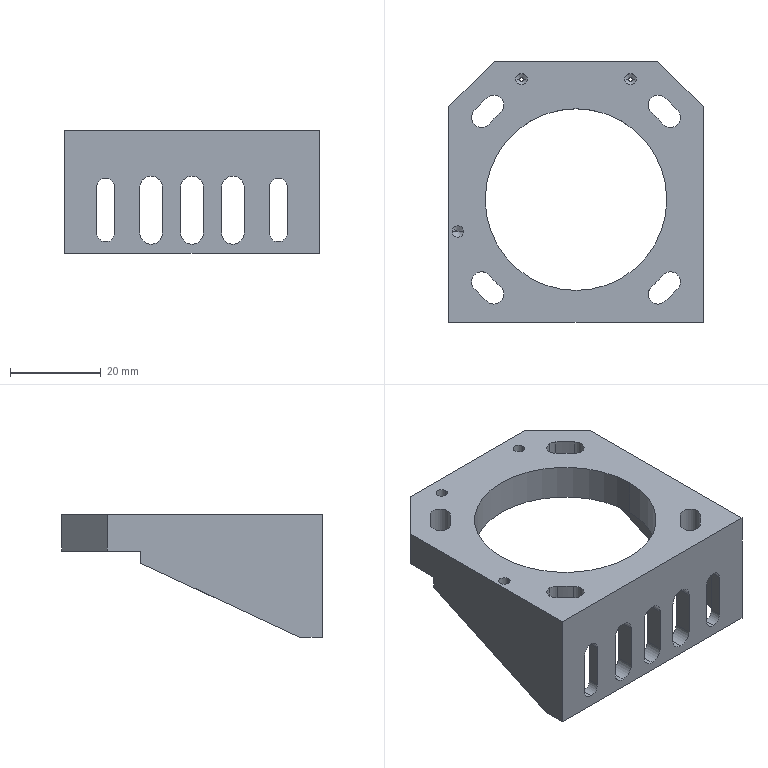NC program | NX | posted with a generic post | part box 56 x 57.4 x 27 mm
Lines 1 to 1144 of 3091:
N10 G17 G21 G94 G90
(ZLEVEL_PROFILE_COPY_1_COPY , TOOL : D3)
N12 T03 M6
N14 G54
N16 G17 G0 G90 X5.642 Y-19.45 B0. C0. S5500 M3
N18 G43 Z30. H3
N20 Z0.8
N22 G94 G1 X9.095 Z0.619 F1000.
N24 X9.326 Y-19.325 Z0.605
N26 X9.45 Y-19.094 Z0.592
N28 Y-18.903 Z0.582
N30 X9.325 Y-18.674 Z0.568
N32 X9.095 Y-18.55 Z0.554
N34 X-1.095 Z0.02
N36 X-1.225 Y-18.599 Z0.013
N38 X-1.335 Y-18.685 Z0.006
N40 X-1.434 Y-18.848 Z-0.004
N42 X-1.448 Y-19.105 Z-0.018
N44 X-1.32 Y-19.33 Z-0.032
N46 X-1.159 Y-19.432 Z-0.042
N48 X-1.095 Y-19.45 Z-0.045
N50 X-1. Z-0.05
N52 X9. F1250.
N54 G3 X9.45 Y-19. R0.45
N56 X9. Y-18.55 R0.45
N58 G1 X-1.
N60 G3 X-1.45 Y-19. R0.45
N62 X-1. Y-19.45 R0.45
N64 G1 X1.864 Z-0.1
N66 X9.
N68 G3 X9.45 Y-19. R0.45
N70 X9. Y-18.55 R0.45
N72 G1 X-1.
N74 G3 X-1.45 Y-19. R0.45
N76 X-1. Y-19.45 R0.45
N78 G1 X1.864 Z-0.15
N80 X9.
N82 G3 X9.45 Y-19. R0.45
N84 X9. Y-18.55 R0.45
N86 G1 X-1.
N88 G3 X-1.45 Y-19. R0.45
N90 X-1. Y-19.45 R0.45
N92 G1 X1.864 Z-0.2
N94 X9.
N96 G3 X9.45 Y-19. R0.45
N98 X9. Y-18.55 R0.45
N100 G1 X-1.
N102 G3 X-1.45 Y-19. R0.45
N104 X-1. Y-19.45 R0.45
N106 G1 X1.864 Z-0.25
N108 X9.
N110 G3 X9.45 Y-19. R0.45
N112 X9. Y-18.55 R0.45
N114 G1 X-1.
N116 G3 X-1.45 Y-19. R0.45
N118 X-1. Y-19.45 R0.45
N120 G1 X1.864 Z-0.3
N122 X9.
N124 G3 X9.45 Y-19. R0.45
N126 X9. Y-18.55 R0.45
N128 G1 X-1.
N130 G3 X-1.45 Y-19. R0.45
N132 X-1. Y-19.45 R0.45
N134 G1 X1.864 Z-0.35
N136 X9.
N138 G3 X9.45 Y-19. R0.45
N140 X9. Y-18.55 R0.45
N142 G1 X-1.
N144 G3 X-1.45 Y-19. R0.45
N146 X-1. Y-19.45 R0.45
N148 G1 X1.864 Z-0.4
N150 X9.
N152 G3 X9.45 Y-19. R0.45
N154 X9. Y-18.55 R0.45
N156 G1 X-1.
N158 G3 X-1.45 Y-19. R0.45
N160 X-1. Y-19.45 R0.45
N162 G1 X1.864 Z-0.45
N164 X9.
N166 G3 X9.45 Y-19. R0.45
N168 X9. Y-18.55 R0.45
N170 G1 X-1.
N172 G3 X-1.45 Y-19. R0.45
N174 X-1. Y-19.45 R0.45
N176 G1 X1.864 Z-0.5
N178 X9.
N180 G3 X9.45 Y-19. R0.45
N182 X9. Y-18.55 R0.45
N184 G1 X-1.
N186 G3 X-1.45 Y-19. R0.45
N188 X-1. Y-19.45 R0.45
N190 G1 X1.864 Z-0.55
N192 X9.
N194 G3 X9.45 Y-19. R0.45
N196 X9. Y-18.55 R0.45
N198 G1 X-1.
N200 G3 X-1.45 Y-19. R0.45
N202 X-1. Y-19.45 R0.45
N204 G1 X1.864 Z-0.6
N206 X9.
N208 G3 X9.45 Y-19. R0.45
N210 X9. Y-18.55 R0.45
N212 G1 X-1.
N214 G3 X-1.45 Y-19. R0.45
N216 X-1. Y-19.45 R0.45
N218 G1 X1.864 Z-0.65
N220 X9.
N222 G3 X9.45 Y-19. R0.45
N224 X9. Y-18.55 R0.45
N226 G1 X-1.
N228 G3 X-1.45 Y-19. R0.45
N230 X-1. Y-19.45 R0.45
N232 G1 X1.864 Z-0.7
N234 X9.
N236 G3 X9.45 Y-19. R0.45
N238 X9. Y-18.55 R0.45
N240 G1 X-1.
N242 G3 X-1.45 Y-19. R0.45
N244 X-1. Y-19.45 R0.45
N246 G1 X1.864 Z-0.75
N248 X9.
N250 G3 X9.45 Y-19. R0.45
N252 X9. Y-18.55 R0.45
N254 G1 X-1.
N256 G3 X-1.45 Y-19. R0.45
N258 X-1. Y-19.45 R0.45
N260 G1 X1.864 Z-0.8
N262 X9.
N264 G3 X9.45 Y-19. R0.45
N266 X9. Y-18.55 R0.45
N268 G1 X-1.
N270 G3 X-1.45 Y-19. R0.45
N272 X-1. Y-19.45 R0.45
N274 G1 X1.864 Z-0.85
N276 X9.
N278 G3 X9.45 Y-19. R0.45
N280 X9. Y-18.55 R0.45
N282 G1 X-1.
N284 G3 X-1.45 Y-19. R0.45
N286 X-1. Y-19.45 R0.45
N288 G1 X1.864 Z-0.9
N290 X9.
N292 G3 X9.45 Y-19. R0.45
N294 X9. Y-18.55 R0.45
N296 G1 X-1.
N298 G3 X-1.45 Y-19. R0.45
N300 X-1. Y-19.45 R0.45
N302 G1 X1.864 Z-0.95
N304 X9.
N306 G3 X9.45 Y-19. R0.45
N308 X9. Y-18.55 R0.45
N310 G1 X-1.
N312 G3 X-1.45 Y-19. R0.45
N314 X-1. Y-19.45 R0.45
N316 G1 X1.864 Z-1.
N318 X9.
N320 G3 X9.45 Y-19. R0.45
N322 X9. Y-18.55 R0.45
N324 G1 X-1.
N326 G3 X-1.45 Y-19. R0.45
N328 X-1. Y-19.45 R0.45
N330 G1 X1.864 Z-1.05
N332 X9.
N334 G3 X9.45 Y-19. R0.45
N336 X9. Y-18.55 R0.45
N338 G1 X-1.
N340 G3 X-1.45 Y-19. R0.45
N342 X-1. Y-19.45 R0.45
N344 G1 X1.864 Z-1.1
N346 X9.
N348 G3 X9.45 Y-19. R0.45
N350 X9. Y-18.55 R0.45
N352 G1 X-1.
N354 G3 X-1.45 Y-19. R0.45
N356 X-1. Y-19.45 R0.45
N358 G1 X1.864 Z-1.15
N360 X9.
N362 G3 X9.45 Y-19. R0.45
N364 X9. Y-18.55 R0.45
N366 G1 X-1.
N368 G3 X-1.45 Y-19. R0.45
N370 X-1. Y-19.45 R0.45
N372 G1 X1.864 Z-1.2
N374 X9.
N376 G3 X9.45 Y-19. R0.45
N378 X9. Y-18.55 R0.45
N380 G1 X-1.
N382 G3 X-1.45 Y-19. R0.45
N384 X-1. Y-19.45 R0.45
N386 G1 X1.864 Z-1.25
N388 X9.
N390 G3 X9.45 Y-19. R0.45
N392 X9. Y-18.55 R0.45
N394 G1 X-1.
N396 G3 X-1.45 Y-19. R0.45
N398 X-1. Y-19.45 R0.45
N400 G1 X1.864 Z-1.3
N402 X9.
N404 G3 X9.45 Y-19. R0.45
N406 X9. Y-18.55 R0.45
N408 G1 X-1.
N410 G3 X-1.45 Y-19. R0.45
N412 X-1. Y-19.45 R0.45
N414 G1 X1.864 Z-1.35
N416 X9.
N418 G3 X9.45 Y-19. R0.45
N420 X9. Y-18.55 R0.45
N422 G1 X-1.
N424 G3 X-1.45 Y-19. R0.45
N426 X-1. Y-19.45 R0.45
N428 G1 X1.864 Z-1.4
N430 X9.
N432 G3 X9.45 Y-19. R0.45
N434 X9. Y-18.55 R0.45
N436 G1 X-1.
N438 G3 X-1.45 Y-19. R0.45
N440 X-1. Y-19.45 R0.45
N442 G1 X1.864 Z-1.45
N444 X9.
N446 G3 X9.45 Y-19. R0.45
N448 X9. Y-18.55 R0.45
N450 G1 X-1.
N452 G3 X-1.45 Y-19. R0.45
N454 X-1. Y-19.45 R0.45
N456 G1 X1.864 Z-1.5
N458 X9.
N460 G3 X9.45 Y-19. R0.45
N462 X9. Y-18.55 R0.45
N464 G1 X-1.
N466 G3 X-1.45 Y-19. R0.45
N468 X-1. Y-19.45 R0.45
N470 G1 X1.864 Z-1.55
N472 X9.
N474 G3 X9.45 Y-19. R0.45
N476 X9. Y-18.55 R0.45
N478 G1 X-1.
N480 G3 X-1.45 Y-19. R0.45
N482 X-1. Y-19.45 R0.45
N484 G1 X1.864 Z-1.6
N486 X9.
N488 G3 X9.45 Y-19. R0.45
N490 X9. Y-18.55 R0.45
N492 G1 X-1.
N494 G3 X-1.45 Y-19. R0.45
N496 X-1. Y-19.45 R0.45
N498 G1 X1.864 Z-1.65
N500 X9.
N502 G3 X9.45 Y-19. R0.45
N504 X9. Y-18.55 R0.45
N506 G1 X-1.
N508 G3 X-1.45 Y-19. R0.45
N510 X-1. Y-19.45 R0.45
N512 G1 X1.864 Z-1.7
N514 X9.
N516 G3 X9.45 Y-19. R0.45
N518 X9. Y-18.55 R0.45
N520 G1 X-1.
N522 G3 X-1.45 Y-19. R0.45
N524 X-1. Y-19.45 R0.45
N526 G1 X1.864 Z-1.75
N528 X9.
N530 G3 X9.45 Y-19. R0.45
N532 X9. Y-18.55 R0.45
N534 G1 X-1.
N536 G3 X-1.45 Y-19. R0.45
N538 X-1. Y-19.45 R0.45
N540 G1 X1.864 Z-1.8
N542 X9.
N544 G3 X9.45 Y-19. R0.45
N546 X9. Y-18.55 R0.45
N548 G1 X-1.
N550 G3 X-1.45 Y-19. R0.45
N552 X-1. Y-19.45 R0.45
N554 G1 X1.864 Z-1.85
N556 X9.
N558 G3 X9.45 Y-19. R0.45
N560 X9. Y-18.55 R0.45
N562 G1 X-1.
N564 G3 X-1.45 Y-19. R0.45
N566 X-1. Y-19.45 R0.45
N568 G1 X1.864 Z-1.9
N570 X9.
N572 G3 X9.45 Y-19. R0.45
N574 X9. Y-18.55 R0.45
N576 G1 X-1.
N578 G3 X-1.45 Y-19. R0.45
N580 X-1. Y-19.45 R0.45
N582 G1 X1.864 Z-1.95
N584 X9.
N586 G3 X9.45 Y-19. R0.45
N588 X9. Y-18.55 R0.45
N590 G1 X-1.
N592 G3 X-1.45 Y-19. R0.45
N594 X-1. Y-19.45 R0.45
N596 G1 X1.864 Z-2.
N598 X9.
N600 G3 X9.45 Y-19. R0.45
N602 X9. Y-18.55 R0.45
N604 G1 X-1.
N606 G3 X-1.45 Y-19. R0.45
N608 X-1. Y-19.45 R0.45
N610 G1 X1.864 Z-2.05
N612 X9.
N614 G3 X9.45 Y-19. R0.45
N616 X9. Y-18.55 R0.45
N618 G1 X-1.
N620 G3 X-1.45 Y-19. R0.45
N622 X-1. Y-19.45 R0.45
N624 G1 X1.864 Z-2.1
N626 X9.
N628 G3 X9.45 Y-19. R0.45
N630 X9. Y-18.55 R0.45
N632 G1 X-1.
N634 G3 X-1.45 Y-19. R0.45
N636 X-1. Y-19.45 R0.45
N638 G1 X1.864 Z-2.15
N640 X9.
N642 G3 X9.45 Y-19. R0.45
N644 X9. Y-18.55 R0.45
N646 G1 X-1.
N648 G3 X-1.45 Y-19. R0.45
N650 X-1. Y-19.45 R0.45
N652 G1 X1.864 Z-2.2
N654 X9.
N656 G3 X9.45 Y-19. R0.45
N658 X9. Y-18.55 R0.45
N660 G1 X-1.
N662 G3 X-1.45 Y-19. R0.45
N664 X-1. Y-19.45 R0.45
N666 G1 X1.864 Z-2.25
N668 X9.
N670 G3 X9.45 Y-19. R0.45
N672 X9. Y-18.55 R0.45
N674 G1 X-1.
N676 G3 X-1.45 Y-19. R0.45
N678 X-1. Y-19.45 R0.45
N680 G1 X1.864 Z-2.3
N682 X9.
N684 G3 X9.45 Y-19. R0.45
N686 X9. Y-18.55 R0.45
N688 G1 X-1.
N690 G3 X-1.45 Y-19. R0.45
N692 X-1. Y-19.45 R0.45
N694 G1 X1.864 Z-2.35
N696 X9.
N698 G3 X9.45 Y-19. R0.45
N700 X9. Y-18.55 R0.45
N702 G1 X-1.
N704 G3 X-1.45 Y-19. R0.45
N706 X-1. Y-19.45 R0.45
N708 G1 X1.864 Z-2.4
N710 X9.
N712 G3 X9.45 Y-19. R0.45
N714 X9. Y-18.55 R0.45
N716 G1 X-1.
N718 G3 X-1.45 Y-19. R0.45
N720 X-1. Y-19.45 R0.45
N722 G1 X1.864 Z-2.45
N724 X9.
N726 G3 X9.45 Y-19. R0.45
N728 X9. Y-18.55 R0.45
N730 G1 X-1.
N732 G3 X-1.45 Y-19. R0.45
N734 X-1. Y-19.45 R0.45
N736 G1 X1.864 Z-2.5
N738 X9.
N740 G3 X9.45 Y-19. R0.45
N742 X9. Y-18.55 R0.45
N744 G1 X-1.
N746 G3 X-1.45 Y-19. R0.45
N748 X-1. Y-19.45 R0.45
N750 G1 X1.864 Z-2.55
N752 X9.
N754 G3 X9.45 Y-19. R0.45
N756 X9. Y-18.55 R0.45
N758 G1 X-1.
N760 G3 X-1.45 Y-19. R0.45
N762 X-1. Y-19.45 R0.45
N764 G1 X1.864 Z-2.6
N766 X9.
N768 G3 X9.45 Y-19. R0.45
N770 X9. Y-18.55 R0.45
N772 G1 X-1.
N774 G3 X-1.45 Y-19. R0.45
N776 X-1. Y-19.45 R0.45
N778 G1 X1.864 Z-2.65
N780 X9.
N782 G3 X9.45 Y-19. R0.45
N784 X9. Y-18.55 R0.45
N786 G1 X-1.
N788 G3 X-1.45 Y-19. R0.45
N790 X-1. Y-19.45 R0.45
N792 G1 X1.864 Z-2.7
N794 X9.
N796 G3 X9.45 Y-19. R0.45
N798 X9. Y-18.55 R0.45
N800 G1 X-1.
N802 G3 X-1.45 Y-19. R0.45
N804 X-1. Y-19.45 R0.45
N806 G1 X1.864 Z-2.75
N808 X9.
N810 G3 X9.45 Y-19. R0.45
N812 X9. Y-18.55 R0.45
N814 G1 X-1.
N816 G3 X-1.45 Y-19. R0.45
N818 X-1. Y-19.45 R0.45
N820 G1 X1.864 Z-2.8
N822 X9.
N824 G3 X9.45 Y-19. R0.45
N826 X9. Y-18.55 R0.45
N828 G1 X-1.
N830 G3 X-1.45 Y-19. R0.45
N832 X-1. Y-19.45 R0.45
N834 G1 X1.864 Z-2.85
N836 X9.
N838 G3 X9.45 Y-19. R0.45
N840 X9. Y-18.55 R0.45
N842 G1 X-1.
N844 G3 X-1.45 Y-19. R0.45
N846 X-1. Y-19.45 R0.45
N848 G1 X1.864 Z-2.9
N850 X9.
N852 G3 X9.45 Y-19. R0.45
N854 X9. Y-18.55 R0.45
N856 G1 X-1.
N858 G3 X-1.45 Y-19. R0.45
N860 X-1. Y-19.45 R0.45
N862 G1 X1.864 Z-2.95
N864 X9.
N866 G3 X9.45 Y-19. R0.45
N868 X9. Y-18.55 R0.45
N870 G1 X-1.
N872 G3 X-1.45 Y-19. R0.45
N874 X-1. Y-19.45 R0.45
N876 G1 X1.864 Z-3.
N878 X9.
N880 G3 X9.45 Y-19. R0.45
N882 X9. Y-18.55 R0.45
N884 G1 X-1.
N886 G3 X-1.45 Y-19. R0.45
N888 X-1. Y-19.45 R0.45
N890 G1 X1.864 Z-3.05
N892 X9.
N894 G3 X9.45 Y-19. R0.45
N896 X9. Y-18.55 R0.45
N898 G1 X-1.
N900 G3 X-1.45 Y-19. R0.45
N902 X-1. Y-19.45 R0.45
N904 G1 X1.864 Z-3.1
N906 X9.
N908 G3 X9.45 Y-19. R0.45
N910 X9. Y-18.55 R0.45
N912 G1 X-1.
N914 G3 X-1.45 Y-19. R0.45
N916 X-1. Y-19.45 R0.45
N918 G1 X1.864 Z-3.15
N920 X9.
N922 G3 X9.45 Y-19. R0.45
N924 X9. Y-18.55 R0.45
N926 G1 X-1.
N928 G3 X-1.45 Y-19. R0.45
N930 X-1. Y-19.45 R0.45
N932 G1 X1.864 Z-3.2
N934 X9.
N936 G3 X9.45 Y-19. R0.45
N938 X9. Y-18.55 R0.45
N940 G1 X-1.
N942 G3 X-1.45 Y-19. R0.45
N944 X-1. Y-19.45 R0.45
N946 G1 X1.864 Z-3.25
N948 X9.
N950 G3 X9.45 Y-19. R0.45
N952 X9. Y-18.55 R0.45
N954 G1 X-1.
N956 G3 X-1.45 Y-19. R0.45
N958 X-1. Y-19.45 R0.45
N960 G1 X1.864 Z-3.3
N962 X9.
N964 G3 X9.45 Y-19. R0.45
N966 X9. Y-18.55 R0.45
N968 G1 X-1.
N970 G3 X-1.45 Y-19. R0.45
N972 X-1. Y-19.45 R0.45
N974 G1 X1.864 Z-3.35
N976 X9.
N978 G3 X9.45 Y-19. R0.45
N980 X9. Y-18.55 R0.45
N982 G1 X-1.
N984 G3 X-1.45 Y-19. R0.45
N986 X-1. Y-19.45 R0.45
N988 G1 X1.864 Z-3.4
N990 X9.
N992 G3 X9.45 Y-19. R0.45
N994 X9. Y-18.55 R0.45
N996 G1 X-1.
N998 G3 X-1.45 Y-19. R0.45
N1000 X-1. Y-19.45 R0.45
N1002 G1 X1.864 Z-3.45
N1004 X9.
N1006 G3 X9.45 Y-19. R0.45
N1008 X9. Y-18.55 R0.45
N1010 G1 X-1.
N1012 G3 X-1.45 Y-19. R0.45
N1014 X-1. Y-19.45 R0.45
N1016 G1 X1.864 Z-3.5
N1018 X9.
N1020 G3 X9.45 Y-19. R0.45
N1022 X9. Y-18.55 R0.45
N1024 G1 X-1.
N1026 G3 X-1.45 Y-19. R0.45
N1028 X-1. Y-19.45 R0.45
N1030 G1 X1.864 Z-3.55
N1032 X9.
N1034 G3 X9.45 Y-19. R0.45
N1036 X9. Y-18.55 R0.45
N1038 G1 X-1.
N1040 G3 X-1.45 Y-19. R0.45
N1042 X-1. Y-19.45 R0.45
N1044 G1 X1.864 Z-3.6
N1046 X9.
N1048 G3 X9.45 Y-19. R0.45
N1050 X9. Y-18.55 R0.45
N1052 G1 X-1.
N1054 G3 X-1.45 Y-19. R0.45
N1056 X-1. Y-19.45 R0.45
N1058 G1 X1.864 Z-3.65
N1060 X9.
N1062 G3 X9.45 Y-19. R0.45
N1064 X9. Y-18.55 R0.45
N1066 G1 X-1.
N1068 G3 X-1.45 Y-19. R0.45
N1070 X-1. Y-19.45 R0.45
N1072 G1 X1.864 Z-3.7
N1074 X9.
N1076 G3 X9.45 Y-19. R0.45
N1078 X9. Y-18.55 R0.45
N1080 G1 X-1.
N1082 G3 X-1.45 Y-19. R0.45
N1084 X-1. Y-19.45 R0.45
N1086 G1 X1.864 Z-3.75
N1088 X9.
N1090 G3 X9.45 Y-19. R0.45
N1092 X9. Y-18.55 R0.45
N1094 G1 X-1.
N1096 G3 X-1.45 Y-19. R0.45
N1098 X-1. Y-19.45 R0.45
N1100 G1 X1.864 Z-3.8
N1102 X9.
N1104 G3 X9.45 Y-19. R0.45
N1106 X9. Y-18.55 R0.45
N1108 G1 X-1.
N1110 G3 X-1.45 Y-19. R0.45
N1112 X-1. Y-19.45 R0.45
N1114 G1 X1.864 Z-3.85
N1116 X9.
N1118 G3 X9.45 Y-19. R0.45
N1120 X9. Y-18.55 R0.45
N1122 G1 X-1.
N1124 G3 X-1.45 Y-19. R0.45
N1126 X-1. Y-19.45 R0.45
N1128 G1 X1.864 Z-3.9
N1130 X9.
N1132 G3 X9.45 Y-19. R0.45
N1134 X9. Y-18.55 R0.45
N1136 G1 X-1.
N1138 G3 X-1.45 Y-19. R0.45
N1140 X-1. Y-19.45 R0.45
N1142 G1 X1.864 Z-3.95
N1144 X9.
N1146 G3 X9.45 Y-19. R0.45
N1148 X9. Y-18.55 R0.45
N1150 G1 X-1.
N1152 G3 X-1.45 Y-19. R0.45
N1154 X-1. Y-19.45 R0.45
N1156 G1 X1.864 Z-4.
N1158 X9.
N1160 G3 X9.45 Y-19. R0.45
N1162 X9. Y-18.55 R0.45
N1164 G1 X-1.
N1166 G3 X-1.45 Y-19. R0.45
N1168 X-1. Y-19.45 R0.45
N1170 G1 X1.864
N1172 Z-3.2
N1174 G0 Z30.
N1176 X8.788 Y-9.95
N1178 Z0.8
N1180 G1 X9.138 Z0.782 F1000.
N1182 X9.432 Y-9.858 Z0.766
N1184 X9.681 Y-9.677 Z0.749
N1186 X9.86 Y-9.427 Z0.733
N1188 X9.951 Y-9.133 Z0.717
N1190 X9.949 Y-8.857 Z0.703
N1192 X9.856 Y-8.566 Z0.687
N1194 X9.677 Y-8.319 Z0.671
N1196 X9.429 Y-8.141 Z0.655
N1198 X9.138 Y-8.05 Z0.639
N1200 X-1.138 Z0.1
N1202 X-1.444 Y-8.149 Z0.083
N1204 X-1.7 Y-8.344 Z0.066
N1206 X-1.878 Y-8.612 Z0.05
N1208 X-1.957 Y-8.924 Z0.033
N1210 X-1.928 Y-9.244 Z0.016
N1212 X-1.82 Y-9.498 Z0.001
N1214 X-1.641 Y-9.714 Z-0.013
N1216 X-1.407 Y-9.869 Z-0.028
N1218 X-1.138 Y-9.95 Z-0.043
N1220 X-1. Z-0.05
N1222 X9. F1250.
N1224 G3 X9.95 Y-9. R0.95
N1226 X9. Y-8.05 R0.95
N1228 G1 X-1.
N1230 G3 X-1.95 Y-9. R0.95
N1232 X-1. Y-9.95 R0.95
N1234 G1 X1.864 Z-0.1
N1236 X9.
N1238 G3 X9.95 Y-9. R0.95
N1240 X9. Y-8.05 R0.95
N1242 G1 X-1.
N1244 G3 X-1.95 Y-9. R0.95
N1246 X-1. Y-9.95 R0.95
N1248 G1 X1.864 Z-0.15
N1250 X9.
N1252 G3 X9.95 Y-9. R0.95
N1254 X9. Y-8.05 R0.95
N1256 G1 X-1.
N1258 G3 X-1.95 Y-9. R0.95
N1260 X-1. Y-9.95 R0.95
N1262 G1 X1.864 Z-0.2
N1264 X9.
N1266 G3 X9.95 Y-9. R0.95
N1268 X9. Y-8.05 R0.95
N1270 G1 X-1.
N1272 G3 X-1.95 Y-9. R0.95
N1274 X-1. Y-9.95 R0.95
N1276 G1 X1.864 Z-0.25
N1278 X9.
N1280 G3 X9.95 Y-9. R0.95
N1282 X9. Y-8.05 R0.95
N1284 G1 X-1.
N1286 G3 X-1.95 Y-9. R0.95
N1288 X-1. Y-9.95 R0.95
N1290 G1 X1.864 Z-0.3
N1292 X9.
N1294 G3 X9.95 Y-9. R0.95
N1296 X9. Y-8.05 R0.95
N1298 G1 X-1.
N1300 G3 X-1.95 Y-9. R0.95
N1302 X-1. Y-9.95 R0.95
N1304 G1 X1.864 Z-0.35
N1306 X9.
N1308 G3 X9.95 Y-9. R0.95
N1310 X9. Y-8.05 R0.95
N1312 G1 X-1.
N1314 G3 X-1.95 Y-9. R0.95
N1316 X-1. Y-9.95 R0.95
N1318 G1 X1.864 Z-0.4
N1320 X9.
N1322 G3 X9.95 Y-9. R0.95
N1324 X9. Y-8.05 R0.95
N1326 G1 X-1.
N1328 G3 X-1.95 Y-9. R0.95
N1330 X-1. Y-9.95 R0.95
N1332 G1 X1.864 Z-0.45
N1334 X9.
N1336 G3 X9.95 Y-9. R0.95
N1338 X9. Y-8.05 R0.95
N1340 G1 X-1.
N1342 G3 X-1.95 Y-9. R0.95
N1344 X-1. Y-9.95 R0.95
N1346 G1 X1.864 Z-0.5
N1348 X9.
N1350 G3 X9.95 Y-9. R0.95
N1352 X9. Y-8.05 R0.95
N1354 G1 X-1.
N1356 G3 X-1.95 Y-9. R0.95
N1358 X-1. Y-9.95 R0.95
N1360 G1 X1.864 Z-0.55
N1362 X9.
N1364 G3 X9.95 Y-9. R0.95
N1366 X9. Y-8.05 R0.95
N1368 G1 X-1.
N1370 G3 X-1.95 Y-9. R0.95
N1372 X-1. Y-9.95 R0.95
N1374 G1 X1.864 Z-0.6
N1376 X9.
N1378 G3 X9.95 Y-9. R0.95
N1380 X9. Y-8.05 R0.95
N1382 G1 X-1.
N1384 G3 X-1.95 Y-9. R0.95
N1386 X-1. Y-9.95 R0.95
N1388 G1 X1.864 Z-0.65
N1390 X9.
N1392 G3 X9.95 Y-9. R0.95
N1394 X9. Y-8.05 R0.95
N1396 G1 X-1.
N1398 G3 X-1.95 Y-9. R0.95
N1400 X-1. Y-9.95 R0.95
N1402 G1 X1.864 Z-0.7
N1404 X9.
N1406 G3 X9.95 Y-9. R0.95
N1408 X9. Y-8.05 R0.95
N1410 G1 X-1.
N1412 G3 X-1.95 Y-9. R0.95
N1414 X-1. Y-9.95 R0.95
N1416 G1 X1.864 Z-0.75
N1418 X9.
N1420 G3 X9.95 Y-9. R0.95
N1422 X9. Y-8.05 R0.95
N1424 G1 X-1.
N1426 G3 X-1.95 Y-9. R0.95
N1428 X-1. Y-9.95 R0.95
N1430 G1 X1.864 Z-0.8
N1432 X9.
N1434 G3 X9.95 Y-9. R0.95
N1436 X9. Y-8.05 R0.95
N1438 G1 X-1.
N1440 G3 X-1.95 Y-9. R0.95
N1442 X-1. Y-9.95 R0.95
N1444 G1 X1.864 Z-0.85
N1446 X9.
N1448 G3 X9.95 Y-9. R0.95
N1450 X9. Y-8.05 R0.95
N1452 G1 X-1.
N1454 G3 X-1.95 Y-9. R0.95
N1456 X-1. Y-9.95 R0.95
N1458 G1 X1.864 Z-0.9
N1460 X9.
N1462 G3 X9.95 Y-9. R0.95
N1464 X9. Y-8.05 R0.95
N1466 G1 X-1.
N1468 G3 X-1.95 Y-9. R0.95
N1470 X-1. Y-9.95 R0.95
N1472 G1 X1.864 Z-0.95
N1474 X9.
N1476 G3 X9.95 Y-9. R0.95
N1478 X9. Y-8.05 R0.95
N1480 G1 X-1.
N1482 G3 X-1.95 Y-9. R0.95
N1484 X-1. Y-9.95 R0.95
N1486 G1 X1.864 Z-1.
N1488 X9.
N1490 G3 X9.95 Y-9. R0.95
N1492 X9. Y-8.05 R0.95
N1494 G1 X-1.
N1496 G3 X-1.95 Y-9. R0.95
N1498 X-1. Y-9.95 R0.95
N1500 G1 X1.864 Z-1.05
N1502 X9.
N1504 G3 X9.95 Y-9. R0.95
N1506 X9. Y-8.05 R0.95
N1508 G1 X-1.
N1510 G3 X-1.95 Y-9. R0.95
N1512 X-1. Y-9.95 R0.95
N1514 G1 X1.864 Z-1.1
N1516 X9.
N1518 G3 X9.95 Y-9. R0.95
N1520 X9. Y-8.05 R0.95
N1522 G1 X-1.
N1524 G3 X-1.95 Y-9. R0.95
N1526 X-1. Y-9.95 R0.95
N1528 G1 X1.864 Z-1.15
N1530 X9.
N1532 G3 X9.95 Y-9. R0.95
N1534 X9. Y-8.05 R0.95
N1536 G1 X-1.
N1538 G3 X-1.95 Y-9. R0.95
N1540 X-1. Y-9.95 R0.95
N1542 G1 X1.864 Z-1.2
N1544 X9.
N1546 G3 X9.95 Y-9. R0.95
N1548 X9. Y-8.05 R0.95
N1550 G1 X-1.
N1552 G3 X-1.95 Y-9. R0.95
N1554 X-1. Y-9.95 R0.95
N1556 G1 X1.864 Z-1.25
N1558 X9.
N1560 G3 X9.95 Y-9. R0.95
N1562 X9. Y-8.05 R0.95
N1564 G1 X-1.
N1566 G3 X-1.95 Y-9. R0.95
N1568 X-1. Y-9.95 R0.95
N1570 G1 X1.864 Z-1.3
N1572 X9.
N1574 G3 X9.95 Y-9. R0.95
N1576 X9. Y-8.05 R0.95
N1578 G1 X-1.
N1580 G3 X-1.95 Y-9. R0.95
N1582 X-1. Y-9.95 R0.95
N1584 G1 X1.864 Z-1.35
N1586 X9.
N1588 G3 X9.95 Y-9. R0.95
N1590 X9. Y-8.05 R0.95
N1592 G1 X-1.
N1594 G3 X-1.95 Y-9. R0.95
N1596 X-1. Y-9.95 R0.95
N1598 G1 X1.864 Z-1.4
N1600 X9.
N1602 G3 X9.95 Y-9. R0.95
N1604 X9. Y-8.05 R0.95
N1606 G1 X-1.
N1608 G3 X-1.95 Y-9. R0.95
N1610 X-1. Y-9.95 R0.95
N1612 G1 X1.864 Z-1.45
N1614 X9.
N1616 G3 X9.95 Y-9. R0.95
N1618 X9. Y-8.05 R0.95
N1620 G1 X-1.
N1622 G3 X-1.95 Y-9. R0.95
N1624 X-1. Y-9.95 R0.95
N1626 G1 X1.864 Z-1.5
N1628 X9.
N1630 G3 X9.95 Y-9. R0.95
N1632 X9. Y-8.05 R0.95
N1634 G1 X-1.
N1636 G3 X-1.95 Y-9. R0.95
N1638 X-1. Y-9.95 R0.95
N1640 G1 X1.864 Z-1.55
N1642 X9.
N1644 G3 X9.95 Y-9. R0.95
N1646 X9. Y-8.05 R0.95
N1648 G1 X-1.
N1650 G3 X-1.95 Y-9. R0.95
N1652 X-1. Y-9.95 R0.95
N1654 G1 X1.864 Z-1.6
N1656 X9.
N1658 G3 X9.95 Y-9. R0.95
N1660 X9. Y-8.05 R0.95
N1662 G1 X-1.
N1664 G3 X-1.95 Y-9. R0.95
N1666 X-1. Y-9.95 R0.95
N1668 G1 X1.864 Z-1.65
N1670 X9.
N1672 G3 X9.95 Y-9. R0.95
N1674 X9. Y-8.05 R0.95
N1676 G1 X-1.
N1678 G3 X-1.95 Y-9. R0.95
N1680 X-1. Y-9.95 R0.95
N1682 G1 X1.864 Z-1.7
N1684 X9.
N1686 G3 X9.95 Y-9. R0.95
N1688 X9. Y-8.05 R0.95
N1690 G1 X-1.
N1692 G3 X-1.95 Y-9. R0.95
N1694 X-1. Y-9.95 R0.95
N1696 G1 X1.864 Z-1.75
N1698 X9.
N1700 G3 X9.95 Y-9. R0.95
N1702 X9. Y-8.05 R0.95
N1704 G1 X-1.
N1706 G3 X-1.95 Y-9. R0.95
N1708 X-1. Y-9.95 R0.95
N1710 G1 X1.864 Z-1.8
N1712 X9.
N1714 G3 X9.95 Y-9. R0.95
N1716 X9. Y-8.05 R0.95
N1718 G1 X-1.
N1720 G3 X-1.95 Y-9. R0.95
N1722 X-1. Y-9.95 R0.95
N1724 G1 X1.864 Z-1.85
N1726 X9.
N1728 G3 X9.95 Y-9. R0.95
N1730 X9. Y-8.05 R0.95
N1732 G1 X-1.
N1734 G3 X-1.95 Y-9. R0.95
N1736 X-1. Y-9.95 R0.95
N1738 G1 X1.864 Z-1.9
N1740 X9.
N1742 G3 X9.95 Y-9. R0.95
N1744 X9. Y-8.05 R0.95
N1746 G1 X-1.
N1748 G3 X-1.95 Y-9. R0.95
N1750 X-1. Y-9.95 R0.95
N1752 G1 X1.864 Z-1.95
N1754 X9.
N1756 G3 X9.95 Y-9. R0.95
N1758 X9. Y-8.05 R0.95
N1760 G1 X-1.
N1762 G3 X-1.95 Y-9. R0.95
N1764 X-1. Y-9.95 R0.95
N1766 G1 X1.864 Z-2.
N1768 X9.
N1770 G3 X9.95 Y-9. R0.95
N1772 X9. Y-8.05 R0.95
N1774 G1 X-1.
N1776 G3 X-1.95 Y-9. R0.95
N1778 X-1. Y-9.95 R0.95
N1780 G1 X1.864 Z-2.05
N1782 X9.
N1784 G3 X9.95 Y-9. R0.95
N1786 X9. Y-8.05 R0.95
N1788 G1 X-1.
N1790 G3 X-1.95 Y-9. R0.95
N1792 X-1. Y-9.95 R0.95
N1794 G1 X1.864 Z-2.1
N1796 X9.
N1798 G3 X9.95 Y-9. R0.95
N1800 X9. Y-8.05 R0.95
N1802 G1 X-1.
N1804 G3 X-1.95 Y-9. R0.95
N1806 X-1. Y-9.95 R0.95
N1808 G1 X1.864 Z-2.15
N1810 X9.
N1812 G3 X9.95 Y-9. R0.95
N1814 X9. Y-8.05 R0.95
N1816 G1 X-1.
N1818 G3 X-1.95 Y-9. R0.95
N1820 X-1. Y-9.95 R0.95
N1822 G1 X1.864 Z-2.2
N1824 X9.
N1826 G3 X9.95 Y-9. R0.95
N1828 X9. Y-8.05 R0.95
N1830 G1 X-1.
N1832 G3 X-1.95 Y-9. R0.95
N1834 X-1. Y-9.95 R0.95
N1836 G1 X1.864 Z-2.25
N1838 X9.
N1840 G3 X9.95 Y-9. R0.95
N1842 X9. Y-8.05 R0.95
N1844 G1 X-1.
N1846 G3 X-1.95 Y-9. R0.95
N1848 X-1. Y-9.95 R0.95
N1850 G1 X1.864 Z-2.3
N1852 X9.
N1854 G3 X9.95 Y-9. R0.95
N1856 X9. Y-8.05 R0.95
N1858 G1 X-1.
N1860 G3 X-1.95 Y-9. R0.95
N1862 X-1. Y-9.95 R0.95
N1864 G1 X1.864 Z-2.35
N1866 X9.
N1868 G3 X9.95 Y-9. R0.95
N1870 X9. Y-8.05 R0.95
N1872 G1 X-1.
N1874 G3 X-1.95 Y-9. R0.95
N1876 X-1. Y-9.95 R0.95
N1878 G1 X1.864 Z-2.4
N1880 X9.
N1882 G3 X9.95 Y-9. R0.95
N1884 X9. Y-8.05 R0.95
N1886 G1 X-1.
N1888 G3 X-1.95 Y-9. R0.95
N1890 X-1. Y-9.95 R0.95
N1892 G1 X1.864 Z-2.45
N1894 X9.
N1896 G3 X9.95 Y-9. R0.95
N1898 X9. Y-8.05 R0.95
N1900 G1 X-1.
N1902 G3 X-1.95 Y-9. R0.95
N1904 X-1. Y-9.95 R0.95
N1906 G1 X1.864 Z-2.5
N1908 X9.
N1910 G3 X9.95 Y-9. R0.95
N1912 X9. Y-8.05 R0.95
N1914 G1 X-1.
N1916 G3 X-1.95 Y-9. R0.95
N1918 X-1. Y-9.95 R0.95
N1920 G1 X1.864 Z-2.55
N1922 X9.
N1924 G3 X9.95 Y-9. R0.95
N1926 X9. Y-8.05 R0.95
N1928 G1 X-1.
N1930 G3 X-1.95 Y-9. R0.95
N1932 X-1. Y-9.95 R0.95
N1934 G1 X1.864 Z-2.6
N1936 X9.
N1938 G3 X9.95 Y-9. R0.95
N1940 X9. Y-8.05 R0.95
N1942 G1 X-1.
N1944 G3 X-1.95 Y-9. R0.95
N1946 X-1. Y-9.95 R0.95
N1948 G1 X1.864 Z-2.65
N1950 X9.
N1952 G3 X9.95 Y-9. R0.95
N1954 X9. Y-8.05 R0.95
N1956 G1 X-1.
N1958 G3 X-1.95 Y-9. R0.95
N1960 X-1. Y-9.95 R0.95
N1962 G1 X1.864 Z-2.7
N1964 X9.
N1966 G3 X9.95 Y-9. R0.95
N1968 X9. Y-8.05 R0.95
N1970 G1 X-1.
N1972 G3 X-1.95 Y-9. R0.95
N1974 X-1. Y-9.95 R0.95
N1976 G1 X1.864 Z-2.75
N1978 X9.
N1980 G3 X9.95 Y-9. R0.95
N1982 X9. Y-8.05 R0.95
N1984 G1 X-1.
N1986 G3 X-1.95 Y-9. R0.95
N1988 X-1. Y-9.95 R0.95
N1990 G1 X1.864 Z-2.8
N1992 X9.
N1994 G3 X9.95 Y-9. R0.95
N1996 X9. Y-8.05 R0.95
N1998 G1 X-1.
N2000 G3 X-1.95 Y-9. R0.95
N2002 X-1. Y-9.95 R0.95
N2004 G1 X1.864 Z-2.85
N2006 X9.
N2008 G3 X9.95 Y-9. R0.95
N2010 X9. Y-8.05 R0.95
N2012 G1 X-1.
N2014 G3 X-1.95 Y-9. R0.95
N2016 X-1. Y-9.95 R0.95
N2018 G1 X1.864 Z-2.9
N2020 X9.
N2022 G3 X9.95 Y-9. R0.95
N2024 X9. Y-8.05 R0.95
N2026 G1 X-1.
N2028 G3 X-1.95 Y-9. R0.95
N2030 X-1. Y-9.95 R0.95
N2032 G1 X1.864 Z-2.95
N2034 X9.
N2036 G3 X9.95 Y-9. R0.95
N2038 X9. Y-8.05 R0.95
N2040 G1 X-1.
N2042 G3 X-1.95 Y-9. R0.95
N2044 X-1. Y-9.95 R0.95
N2046 G1 X1.864 Z-3.
N2048 X9.
N2050 G3 X9.95 Y-9. R0.95
N2052 X9. Y-8.05 R0.95
N2054 G1 X-1.
N2056 G3 X-1.95 Y-9. R0.95
N2058 X-1. Y-9.95 R0.95
N2060 G1 X1.864 Z-3.05
N2062 X9.
N2064 G3 X9.95 Y-9. R0.95
N2066 X9. Y-8.05 R0.95
N2068 G1 X-1.
N2070 G3 X-1.95 Y-9. R0.95
N2072 X-1. Y-9.95 R0.95
N2074 G1 X1.864 Z-3.1
N2076 X9.
N2078 G3 X9.95 Y-9. R0.95
N2080 X9. Y-8.05 R0.95
N2082 G1 X-1.
N2084 G3 X-1.95 Y-9. R0.95
N2086 X-1. Y-9.95 R0.95
N2088 G1 X1.864 Z-3.15
N2090 X9.
N2092 G3 X9.95 Y-9. R0.95
N2094 X9. Y-8.05 R0.95
N2096 G1 X-1.
N2098 G3 X-1.95 Y-9. R0.95
N2100 X-1. Y-9.95 R0.95
N2102 G1 X1.864 Z-3.2
N2104 X9.
N2106 G3 X9.95 Y-9. R0.95
N2108 X9. Y-8.05 R0.95
N2110 G1 X-1.
N2112 G3 X-1.95 Y-9. R0.95
N2114 X-1. Y-9.95 R0.95
N2116 G1 X1.864 Z-3.25
N2118 X9.
N2120 G3 X9.95 Y-9. R0.95
N2122 X9. Y-8.05 R0.95
N2124 G1 X-1.
N2126 G3 X-1.95 Y-9. R0.95
N2128 X-1. Y-9.95 R0.95
N2130 G1 X1.864 Z-3.3
N2132 X9.
N2134 G3 X9.95 Y-9. R0.95
N2136 X9. Y-8.05 R0.95
N2138 G1 X-1.
N2140 G3 X-1.95 Y-9. R0.95
N2142 X-1. Y-9.95 R0.95
N2144 G1 X1.864 Z-3.35
N2146 X9.
N2148 G3 X9.95 Y-9. R0.95
N2150 X9. Y-8.05 R0.95
N2152 G1 X-1.
N2154 G3 X-1.95 Y-9. R0.95
N2156 X-1. Y-9.95 R0.95
N2158 G1 X1.864 Z-3.4
N2160 X9.
N2162 G3 X9.95 Y-9. R0.95
N2164 X9. Y-8.05 R0.95
N2166 G1 X-1.
N2168 G3 X-1.95 Y-9. R0.95
N2170 X-1. Y-9.95 R0.95
N2172 G1 X1.864 Z-3.45
N2174 X9.
N2176 G3 X9.95 Y-9. R0.95
N2178 X9. Y-8.05 R0.95
N2180 G1 X-1.
N2182 G3 X-1.95 Y-9. R0.95
N2184 X-1. Y-9.95 R0.95
N2186 G1 X1.864 Z-3.5
N2188 X9.
N2190 G3 X9.95 Y-9. R0.95
N2192 X9. Y-8.05 R0.95
N2194 G1 X-1.
N2196 G3 X-1.95 Y-9. R0.95
N2198 X-1. Y-9.95 R0.95
N2200 G1 X1.864 Z-3.55
N2202 X9.
N2204 G3 X9.95 Y-9. R0.95
N2206 X9. Y-8.05 R0.95
N2208 G1 X-1.
N2210 G3 X-1.95 Y-9. R0.95
N2212 X-1. Y-9.95 R0.95
N2214 G1 X1.864 Z-3.6
N2216 X9.
N2218 G3 X9.95 Y-9. R0.95
N2220 X9. Y-8.05 R0.95
N2222 G1 X-1.
N2224 G3 X-1.95 Y-9. R0.95
N2226 X-1. Y-9.95 R0.95
N2228 G1 X1.864 Z-3.65
N2230 X9.
N2232 G3 X9.95 Y-9. R0.95
N2234 X9. Y-8.05 R0.95
N2236 G1 X-1.
N2238 G3 X-1.95 Y-9. R0.95
N2240 X-1. Y-9.95 R0.95
N2242 G1 X1.864 Z-3.7
N2244 X9.
N2246 G3 X9.95 Y-9. R0.95
N2248 X9. Y-8.05 R0.95
N2250 G1 X-1.
N2252 G3 X-1.95 Y-9. R0.95
N2254 X-1. Y-9.95 R0.95
N2256 G1 X1.864 Z-3.75
N2258 X9.
N2260 G3 X9.95 Y-9. R0.95
N2262 X9. Y-8.05 R0.95
N2264 G1 X-1.
N2266 G3 X-1.95 Y-9. R0.95
N2268 X-1. Y-9.95 R0.95
N2270 G1 X1.864 Z-3.8
N2272 X9.
N2274 G3 X9.95 Y-9. R0.95
N2276 X9. Y-8.05 R0.95
N2278 G1 X-1.
N2280 G3 X-1.95 Y-9. R0.95
N2282 X-1. Y-9.95 R0.95
N2284 G1 X1.864 Z-3.85
N2286 X9.